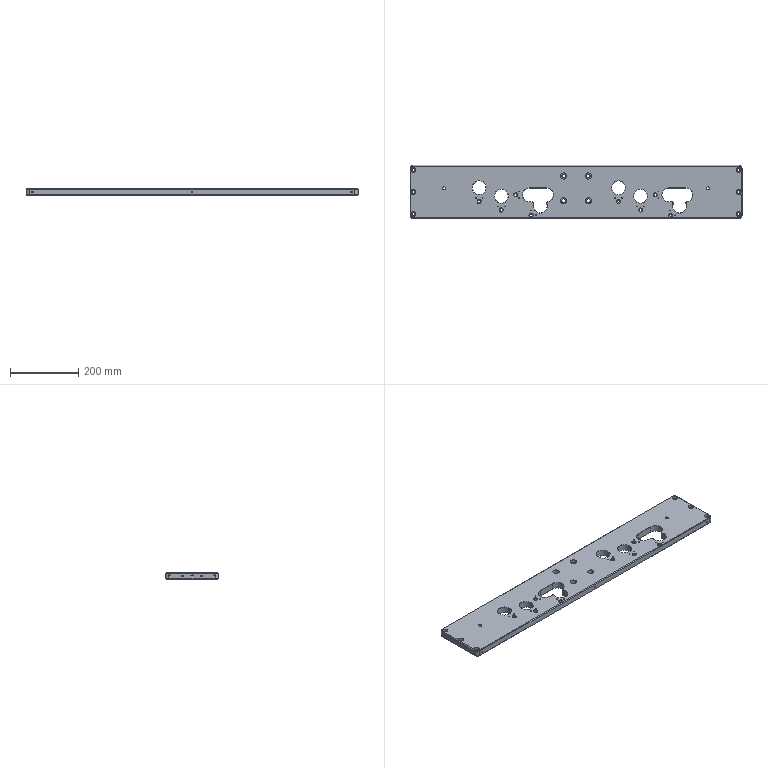Part | SolidWorks | features Chamfer 10, 3DProfileFeature 8, HoleWzd 8, ICE 8, LPattern 6, Fillet 3, Extrusion 1 | 1 solid | 404 faces | box 970 x 155 x 20 mm | volume 2656838 mm3 | cone 186 | cylinder 180 | plane 38 | commonest cylinder face diameters 4.2 x36 2.5 x32 5 x20 40 x20 8 x16 9 x16